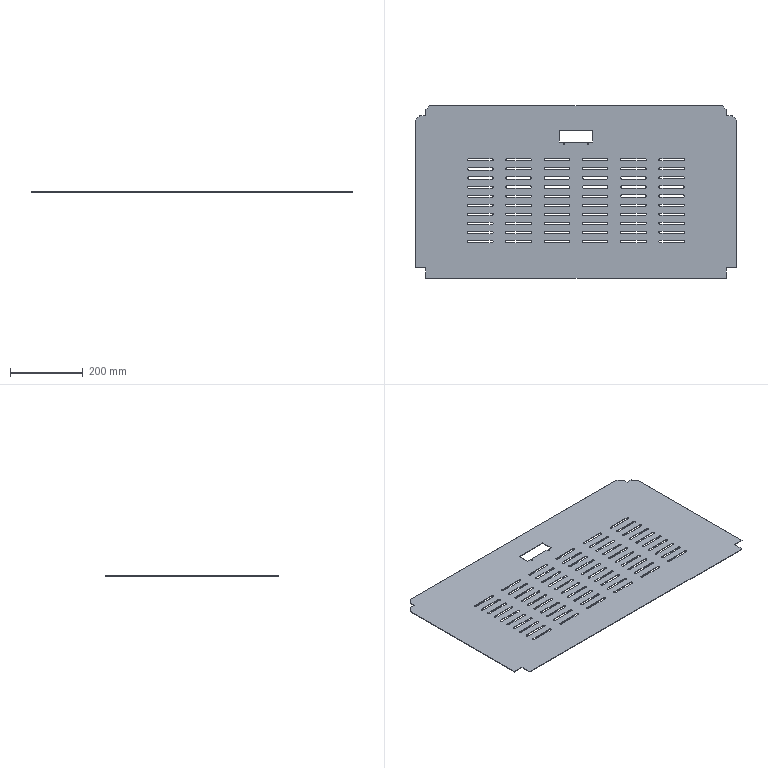Part | STEP file | Left Side Panel Closing Plate | 1 solid | 284 faces | box 885.969 x 475.969 x 1.5 mm | volume 584980 mm3 | plane 158 | cylinder 126 | commonest cylinder face diameters 6 x122 3.2 x4